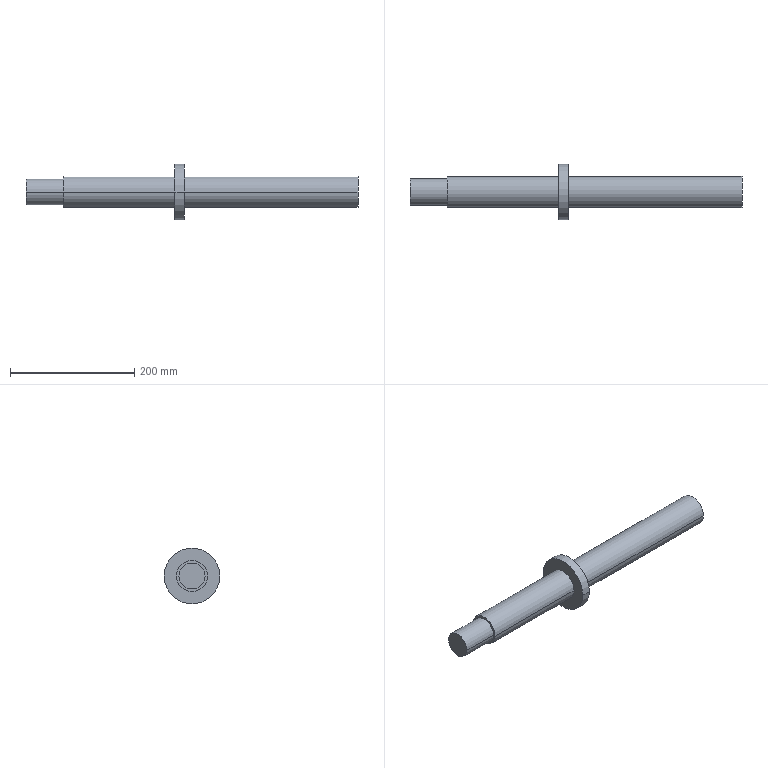Part | SolidWorks | features ICE 2, Revolution 1 | 1 solid | 13 faces | box 535 x 90 x 90 mm | volume 1081760 mm3 | cylinder 8 | plane 5 | commonest cylinder face diameters 50 x4 42 x2 90 x2
STEP:
#1=CARTESIAN_POINT('',(-247.5,-21.,0.));
#2=VERTEX_POINT('',#1);
#3=CARTESIAN_POINT('',(-247.5,21.,0.));
#4=VERTEX_POINT('',#3);
#5=CARTESIAN_POINT('',(-247.5,0.,0.));
#6=DIRECTION('',(-1.,0.,0.));
#7=DIRECTION('',(0.,-1.,0.));
#8=AXIS2_PLACEMENT_3D('',#5,#6,#7);
#9=CIRCLE('',#8,21.);
#10=EDGE_CURVE('',#2,#4,#9,.T.);
#11=ORIENTED_EDGE('',*,*,#10,.F.);
#12=CARTESIAN_POINT('',(-187.5,-21.,0.));
#13=VERTEX_POINT('',#12);
#14=CARTESIAN_POINT('',(-247.5,-21.,0.));
#15=DIRECTION('',(1.,0.,0.));
#16=VECTOR('',#15,1000.);
#17=LINE('',#14,#16);
#18=EDGE_CURVE('',#2,#13,#17,.T.);
#19=ORIENTED_EDGE('',*,*,#18,.T.);
#20=CARTESIAN_POINT('',(-187.5,21.,0.));
#21=VERTEX_POINT('',#20);
#22=CARTESIAN_POINT('',(-187.5,0.,0.));
#23=DIRECTION('',(-1.,0.,0.));
#24=DIRECTION('',(0.,-1.,0.));
#25=AXIS2_PLACEMENT_3D('',#22,#23,#24);
#26=CIRCLE('',#25,21.);
#27=EDGE_CURVE('',#13,#21,#26,.T.);
#28=ORIENTED_EDGE('',*,*,#27,.T.);
#29=CARTESIAN_POINT('',(-247.5,21.,0.));
#30=DIRECTION('',(1.,0.,0.));
#31=VECTOR('',#30,1000.);
#32=LINE('',#29,#31);
#33=EDGE_CURVE('',#4,#21,#32,.T.);
#34=ORIENTED_EDGE('',*,*,#33,.F.);
#35=EDGE_LOOP('',(#11,#19,#28,#34));
#36=FACE_OUTER_BOUND('',#35,.T.);
#37=CARTESIAN_POINT('',(-247.5,0.,0.));
#38=DIRECTION('',(1.,0.,0.));
#39=DIRECTION('',(0.,1.,0.));
#40=AXIS2_PLACEMENT_3D('',#37,#38,#39);
#41=CYLINDRICAL_SURFACE('',#40,21.);
#42=ADVANCED_FACE('',(#36),#41,.T.);
#43=CARTESIAN_POINT('',(-7.5,-25.,0.));
#44=VERTEX_POINT('',#43);
#45=CARTESIAN_POINT('',(-7.5,25.,0.));
#46=VERTEX_POINT('',#45);
#47=CARTESIAN_POINT('',(-7.5,0.,0.));
#48=DIRECTION('',(-1.,0.,0.));
#49=DIRECTION('',(0.,-1.,0.));
#50=AXIS2_PLACEMENT_3D('',#47,#48,#49);
#51=CIRCLE('',#50,25.);
#52=EDGE_CURVE('',#44,#46,#51,.T.);
#53=ORIENTED_EDGE('',*,*,#52,.T.);
#54=CARTESIAN_POINT('',(-187.5,25.,0.));
#55=VERTEX_POINT('',#54);
#56=CARTESIAN_POINT('',(-187.5,25.,0.));
#57=DIRECTION('',(-1.,0.,0.));
#58=VECTOR('',#57,1000.);
#59=LINE('',#56,#58);
#60=EDGE_CURVE('',#46,#55,#59,.T.);
#61=ORIENTED_EDGE('',*,*,#60,.T.);
#62=CARTESIAN_POINT('',(-187.5,-25.,0.));
#63=VERTEX_POINT('',#62);
#64=CARTESIAN_POINT('',(-187.5,0.,0.));
#65=DIRECTION('',(-1.,0.,0.));
#66=DIRECTION('',(0.,-1.,0.));
#67=AXIS2_PLACEMENT_3D('',#64,#65,#66);
#68=CIRCLE('',#67,25.);
#69=EDGE_CURVE('',#63,#55,#68,.T.);
#70=ORIENTED_EDGE('',*,*,#69,.F.);
#71=CARTESIAN_POINT('',(-187.5,-25.,0.));
#72=DIRECTION('',(-1.,0.,0.));
#73=VECTOR('',#72,1000.);
#74=LINE('',#71,#73);
#75=EDGE_CURVE('',#44,#63,#74,.T.);
#76=ORIENTED_EDGE('',*,*,#75,.F.);
#77=EDGE_LOOP('',(#53,#61,#70,#76));
#78=FACE_OUTER_BOUND('',#77,.T.);
#79=CARTESIAN_POINT('',(-187.5,0.,0.));
#80=DIRECTION('',(-1.,0.,0.));
#81=DIRECTION('',(0.,-1.,0.));
#82=AXIS2_PLACEMENT_3D('',#79,#80,#81);
#83=CYLINDRICAL_SURFACE('',#82,25.);
#84=ADVANCED_FACE('',(#78),#83,.T.);
#85=CARTESIAN_POINT('',(7.5,-45.,0.));
#86=VERTEX_POINT('',#85);
#87=CARTESIAN_POINT('',(7.5,45.,0.));
#88=VERTEX_POINT('',#87);
#89=CARTESIAN_POINT('',(7.5,0.,0.));
#90=DIRECTION('',(-1.,0.,0.));
#91=DIRECTION('',(0.,-1.,0.));
#92=AXIS2_PLACEMENT_3D('',#89,#90,#91);
#93=CIRCLE('',#92,45.);
#94=EDGE_CURVE('',#86,#88,#93,.T.);
#95=ORIENTED_EDGE('',*,*,#94,.T.);
#96=CARTESIAN_POINT('',(-7.5,45.,0.));
#97=VERTEX_POINT('',#96);
#98=CARTESIAN_POINT('',(-187.5,45.,0.));
#99=DIRECTION('',(-1.,0.,0.));
#100=VECTOR('',#99,1000.);
#101=LINE('',#98,#100);
#102=EDGE_CURVE('',#88,#97,#101,.T.);
#103=ORIENTED_EDGE('',*,*,#102,.T.);
#104=CARTESIAN_POINT('',(-7.5,-45.,0.));
#105=VERTEX_POINT('',#104);
#106=CARTESIAN_POINT('',(-7.5,0.,0.));
#107=DIRECTION('',(-1.,0.,0.));
#108=DIRECTION('',(0.,-1.,0.));
#109=AXIS2_PLACEMENT_3D('',#106,#107,#108);
#110=CIRCLE('',#109,45.);
#111=EDGE_CURVE('',#105,#97,#110,.T.);
#112=ORIENTED_EDGE('',*,*,#111,.F.);
#113=CARTESIAN_POINT('',(-187.5,-45.,0.));
#114=DIRECTION('',(-1.,0.,0.));
#115=VECTOR('',#114,1000.);
#116=LINE('',#113,#115);
#117=EDGE_CURVE('',#86,#105,#116,.T.);
#118=ORIENTED_EDGE('',*,*,#117,.F.);
#119=EDGE_LOOP('',(#95,#103,#112,#118));
#120=FACE_OUTER_BOUND('',#119,.T.);
#121=CARTESIAN_POINT('',(-187.5,0.,0.));
#122=DIRECTION('',(-1.,0.,0.));
#123=DIRECTION('',(0.,-1.,0.));
#124=AXIS2_PLACEMENT_3D('',#121,#122,#123);
#125=CYLINDRICAL_SURFACE('',#124,45.);
#126=ADVANCED_FACE('',(#120),#125,.T.);
#127=CARTESIAN_POINT('',(287.5,25.,0.));
#128=VERTEX_POINT('',#127);
#129=CARTESIAN_POINT('',(287.5,-25.,0.));
#130=VERTEX_POINT('',#129);
#131=CARTESIAN_POINT('',(287.5,0.,0.));
#132=DIRECTION('',(1.,0.,0.));
#133=DIRECTION('',(0.,1.,0.));
#134=AXIS2_PLACEMENT_3D('',#131,#132,#133);
#135=CIRCLE('',#134,25.);
#136=EDGE_CURVE('',#128,#130,#135,.T.);
#137=ORIENTED_EDGE('',*,*,#136,.F.);
#138=CARTESIAN_POINT('',(7.5,25.,0.));
#139=VERTEX_POINT('',#138);
#140=CARTESIAN_POINT('',(-187.5,25.,0.));
#141=DIRECTION('',(-1.,0.,0.));
#142=VECTOR('',#141,1000.);
#143=LINE('',#140,#142);
#144=EDGE_CURVE('',#128,#139,#143,.T.);
#145=ORIENTED_EDGE('',*,*,#144,.T.);
#146=CARTESIAN_POINT('',(7.5,-25.,0.));
#147=VERTEX_POINT('',#146);
#148=CARTESIAN_POINT('',(7.5,0.,0.));
#149=DIRECTION('',(-1.,0.,0.));
#150=DIRECTION('',(0.,-1.,0.));
#151=AXIS2_PLACEMENT_3D('',#148,#149,#150);
#152=CIRCLE('',#151,25.);
#153=EDGE_CURVE('',#147,#139,#152,.T.);
#154=ORIENTED_EDGE('',*,*,#153,.F.);
#155=CARTESIAN_POINT('',(-187.5,-25.,0.));
#156=DIRECTION('',(-1.,0.,0.));
#157=VECTOR('',#156,1000.);
#158=LINE('',#155,#157);
#159=EDGE_CURVE('',#130,#147,#158,.T.);
#160=ORIENTED_EDGE('',*,*,#159,.F.);
#161=EDGE_LOOP('',(#137,#145,#154,#160));
#162=FACE_OUTER_BOUND('',#161,.T.);
#163=CARTESIAN_POINT('',(-187.5,0.,0.));
#164=DIRECTION('',(-1.,0.,0.));
#165=DIRECTION('',(0.,-1.,0.));
#166=AXIS2_PLACEMENT_3D('',#163,#164,#165);
#167=CYLINDRICAL_SURFACE('',#166,25.);
#168=ADVANCED_FACE('',(#162),#167,.T.);
#169=ORIENTED_EDGE('',*,*,#144,.F.);
#170=CARTESIAN_POINT('',(287.5,0.,0.));
#171=DIRECTION('',(1.,0.,0.));
#172=DIRECTION('',(0.,1.,0.));
#173=AXIS2_PLACEMENT_3D('',#170,#171,#172);
#174=CIRCLE('',#173,25.);
#175=EDGE_CURVE('',#130,#128,#174,.T.);
#176=ORIENTED_EDGE('',*,*,#175,.F.);
#177=ORIENTED_EDGE('',*,*,#159,.T.);
#178=CARTESIAN_POINT('',(7.5,0.,0.));
#179=DIRECTION('',(-1.,0.,0.));
#180=DIRECTION('',(0.,-1.,0.));
#181=AXIS2_PLACEMENT_3D('',#178,#179,#180);
#182=CIRCLE('',#181,25.);
#183=EDGE_CURVE('',#139,#147,#182,.T.);
#184=ORIENTED_EDGE('',*,*,#183,.F.);
#185=EDGE_LOOP('',(#169,#176,#177,#184));
#186=FACE_OUTER_BOUND('',#185,.T.);
#187=CARTESIAN_POINT('',(-187.5,0.,0.));
#188=DIRECTION('',(-1.,0.,0.));
#189=DIRECTION('',(0.,-1.,0.));
#190=AXIS2_PLACEMENT_3D('',#187,#188,#189);
#191=CYLINDRICAL_SURFACE('',#190,25.);
#192=ADVANCED_FACE('',(#186),#191,.T.);
#193=ORIENTED_EDGE('',*,*,#94,.F.);
#194=CARTESIAN_POINT('',(7.5,0.,0.));
#195=DIRECTION('',(-1.,0.,0.));
#196=DIRECTION('',(0.,-1.,0.));
#197=AXIS2_PLACEMENT_3D('',#194,#195,#196);
#198=CIRCLE('',#197,45.);
#199=EDGE_CURVE('',#88,#86,#198,.T.);
#200=ORIENTED_EDGE('',*,*,#199,.F.);
#201=EDGE_LOOP('',(#193,#200));
#202=FACE_OUTER_BOUND('',#201,.T.);
#203=ORIENTED_EDGE('',*,*,#153,.T.);
#204=ORIENTED_EDGE('',*,*,#183,.T.);
#205=EDGE_LOOP('',(#203,#204));
#206=FACE_BOUND('',#205,.T.);
#207=CARTESIAN_POINT('',(7.5,25.,0.));
#208=DIRECTION('',(-1.,0.,0.));
#209=DIRECTION('',(0.,-1.,0.));
#210=AXIS2_PLACEMENT_3D('',#207,#208,#209);
#211=PLANE('',#210);
#212=ADVANCED_FACE('',(#202,#206),#211,.F.);
#213=ORIENTED_EDGE('',*,*,#102,.F.);
#214=ORIENTED_EDGE('',*,*,#199,.T.);
#215=ORIENTED_EDGE('',*,*,#117,.T.);
#216=CARTESIAN_POINT('',(-7.5,0.,0.));
#217=DIRECTION('',(-1.,0.,0.));
#218=DIRECTION('',(0.,-1.,0.));
#219=AXIS2_PLACEMENT_3D('',#216,#217,#218);
#220=CIRCLE('',#219,45.);
#221=EDGE_CURVE('',#97,#105,#220,.T.);
#222=ORIENTED_EDGE('',*,*,#221,.F.);
#223=EDGE_LOOP('',(#213,#214,#215,#222));
#224=FACE_OUTER_BOUND('',#223,.T.);
#225=CARTESIAN_POINT('',(-187.5,0.,0.));
#226=DIRECTION('',(-1.,0.,0.));
#227=DIRECTION('',(0.,-1.,0.));
#228=AXIS2_PLACEMENT_3D('',#225,#226,#227);
#229=CYLINDRICAL_SURFACE('',#228,45.);
#230=ADVANCED_FACE('',(#224),#229,.T.);
#231=ORIENTED_EDGE('',*,*,#52,.F.);
#232=CARTESIAN_POINT('',(-7.5,0.,0.));
#233=DIRECTION('',(-1.,0.,0.));
#234=DIRECTION('',(0.,-1.,0.));
#235=AXIS2_PLACEMENT_3D('',#232,#233,#234);
#236=CIRCLE('',#235,25.);
#237=EDGE_CURVE('',#46,#44,#236,.T.);
#238=ORIENTED_EDGE('',*,*,#237,.F.);
#239=EDGE_LOOP('',(#231,#238));
#240=FACE_BOUND('',#239,.T.);
#241=ORIENTED_EDGE('',*,*,#111,.T.);
#242=ORIENTED_EDGE('',*,*,#221,.T.);
#243=EDGE_LOOP('',(#241,#242));
#244=FACE_OUTER_BOUND('',#243,.T.);
#245=CARTESIAN_POINT('',(-7.5,25.,0.));
#246=DIRECTION('',(1.,0.,0.));
#247=DIRECTION('',(0.,1.,0.));
#248=AXIS2_PLACEMENT_3D('',#245,#246,#247);
#249=PLANE('',#248);
#250=ADVANCED_FACE('',(#240,#244),#249,.F.);
#251=ORIENTED_EDGE('',*,*,#60,.F.);
#252=ORIENTED_EDGE('',*,*,#237,.T.);
#253=ORIENTED_EDGE('',*,*,#75,.T.);
#254=CARTESIAN_POINT('',(-187.5,0.,0.));
#255=DIRECTION('',(-1.,0.,0.));
#256=DIRECTION('',(0.,-1.,0.));
#257=AXIS2_PLACEMENT_3D('',#254,#255,#256);
#258=CIRCLE('',#257,25.);
#259=EDGE_CURVE('',#55,#63,#258,.T.);
#260=ORIENTED_EDGE('',*,*,#259,.F.);
#261=EDGE_LOOP('',(#251,#252,#253,#260));
#262=FACE_OUTER_BOUND('',#261,.T.);
#263=CARTESIAN_POINT('',(-187.5,0.,0.));
#264=DIRECTION('',(-1.,0.,0.));
#265=DIRECTION('',(0.,-1.,0.));
#266=AXIS2_PLACEMENT_3D('',#263,#264,#265);
#267=CYLINDRICAL_SURFACE('',#266,25.);
#268=ADVANCED_FACE('',(#262),#267,.T.);
#269=CARTESIAN_POINT('',(-187.5,0.,0.));
#270=DIRECTION('',(-1.,0.,0.));
#271=DIRECTION('',(0.,-1.,0.));
#272=AXIS2_PLACEMENT_3D('',#269,#270,#271);
#273=CIRCLE('',#272,21.);
#274=EDGE_CURVE('',#21,#13,#273,.T.);
#275=ORIENTED_EDGE('',*,*,#274,.F.);
#276=ORIENTED_EDGE('',*,*,#27,.F.);
#277=EDGE_LOOP('',(#275,#276));
#278=FACE_BOUND('',#277,.T.);
#279=ORIENTED_EDGE('',*,*,#69,.T.);
#280=ORIENTED_EDGE('',*,*,#259,.T.);
#281=EDGE_LOOP('',(#279,#280));
#282=FACE_OUTER_BOUND('',#281,.T.);
#283=CARTESIAN_POINT('',(-187.5,0.,0.));
#284=DIRECTION('',(1.,0.,0.));
#285=DIRECTION('',(0.,1.,0.));
#286=AXIS2_PLACEMENT_3D('',#283,#284,#285);
#287=PLANE('',#286);
#288=ADVANCED_FACE('',(#278,#282),#287,.F.);
#289=ORIENTED_EDGE('',*,*,#175,.T.);
#290=ORIENTED_EDGE('',*,*,#136,.T.);
#291=EDGE_LOOP('',(#289,#290));
#292=FACE_OUTER_BOUND('',#291,.T.);
#293=CARTESIAN_POINT('',(287.5,0.,0.));
#294=DIRECTION('',(1.,0.,0.));
#295=DIRECTION('',(0.,1.,0.));
#296=AXIS2_PLACEMENT_3D('',#293,#294,#295);
#297=PLANE('',#296);
#298=ADVANCED_FACE('',(#292),#297,.T.);
#299=ORIENTED_EDGE('',*,*,#18,.F.);
#300=CARTESIAN_POINT('',(-247.5,0.,0.));
#301=DIRECTION('',(-1.,0.,0.));
#302=DIRECTION('',(0.,-1.,0.));
#303=AXIS2_PLACEMENT_3D('',#300,#301,#302);
#304=CIRCLE('',#303,21.);
#305=EDGE_CURVE('',#4,#2,#304,.T.);
#306=ORIENTED_EDGE('',*,*,#305,.F.);
#307=ORIENTED_EDGE('',*,*,#33,.T.);
#308=ORIENTED_EDGE('',*,*,#274,.T.);
#309=EDGE_LOOP('',(#299,#306,#307,#308));
#310=FACE_OUTER_BOUND('',#309,.T.);
#311=CARTESIAN_POINT('',(-247.5,0.,0.));
#312=DIRECTION('',(1.,0.,0.));
#313=DIRECTION('',(0.,1.,0.));
#314=AXIS2_PLACEMENT_3D('',#311,#312,#313);
#315=CYLINDRICAL_SURFACE('',#314,21.);
#316=ADVANCED_FACE('',(#310),#315,.T.);
#317=ORIENTED_EDGE('',*,*,#305,.T.);
#318=ORIENTED_EDGE('',*,*,#10,.T.);
#319=EDGE_LOOP('',(#317,#318));
#320=FACE_OUTER_BOUND('',#319,.T.);
#321=CARTESIAN_POINT('',(-247.5,0.,0.));
#322=DIRECTION('',(-1.,0.,0.));
#323=DIRECTION('',(0.,-1.,0.));
#324=AXIS2_PLACEMENT_3D('',#321,#322,#323);
#325=PLANE('',#324);
#326=ADVANCED_FACE('',(#320),#325,.T.);
#327=CLOSED_SHELL('',(#42,#84,#126,#168,#192,#212,#230,#250,#268,#288,#298,#316,#326));
#328=MANIFOLD_SOLID_BREP('',#327);
#329=CARTESIAN_POINT('',(0.,0.,0.));
#330=DIRECTION('',(0.,0.,1.));
#331=DIRECTION('',(1.,0.,0.));
#332=AXIS2_PLACEMENT_3D('',#329,#330,#331);
#333=(LENGTH_UNIT()NAMED_UNIT(*)SI_UNIT(.MILLI.,.METRE.));
#334=UNCERTAINTY_MEASURE_WITH_UNIT(LENGTH_MEASURE(0.00001),#333,'','');
#335=(NAMED_UNIT(*)PLANE_ANGLE_UNIT()SI_UNIT($,.RADIAN.));
#336=(NAMED_UNIT(*)SI_UNIT($,.STERADIAN.)SOLID_ANGLE_UNIT());
#337=(GEOMETRIC_REPRESENTATION_CONTEXT(3)GLOBAL_UNCERTAINTY_ASSIGNED_CONTEXT((#334))GLOBAL_UNIT_ASSIGNED_CONTEXT((#333,#335,#336))REPRESENTATION_CONTEXT('',''));
#338=ADVANCED_BREP_SHAPE_REPRESENTATION('',(#328,#332),#337);